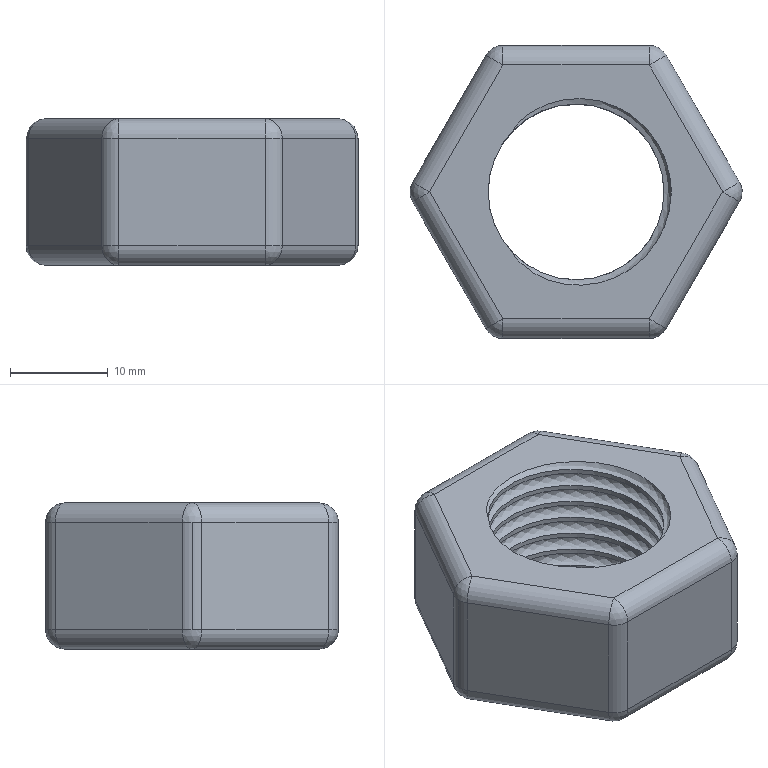Part | SolidWorks | features BaseBody 1 | 1 solid | 57 faces | volume 7321 mm3 | cylinder 35 | sphere 12 | plane 9 | spline 1 | commonest cylinder face diameters 4 x19 18 x16